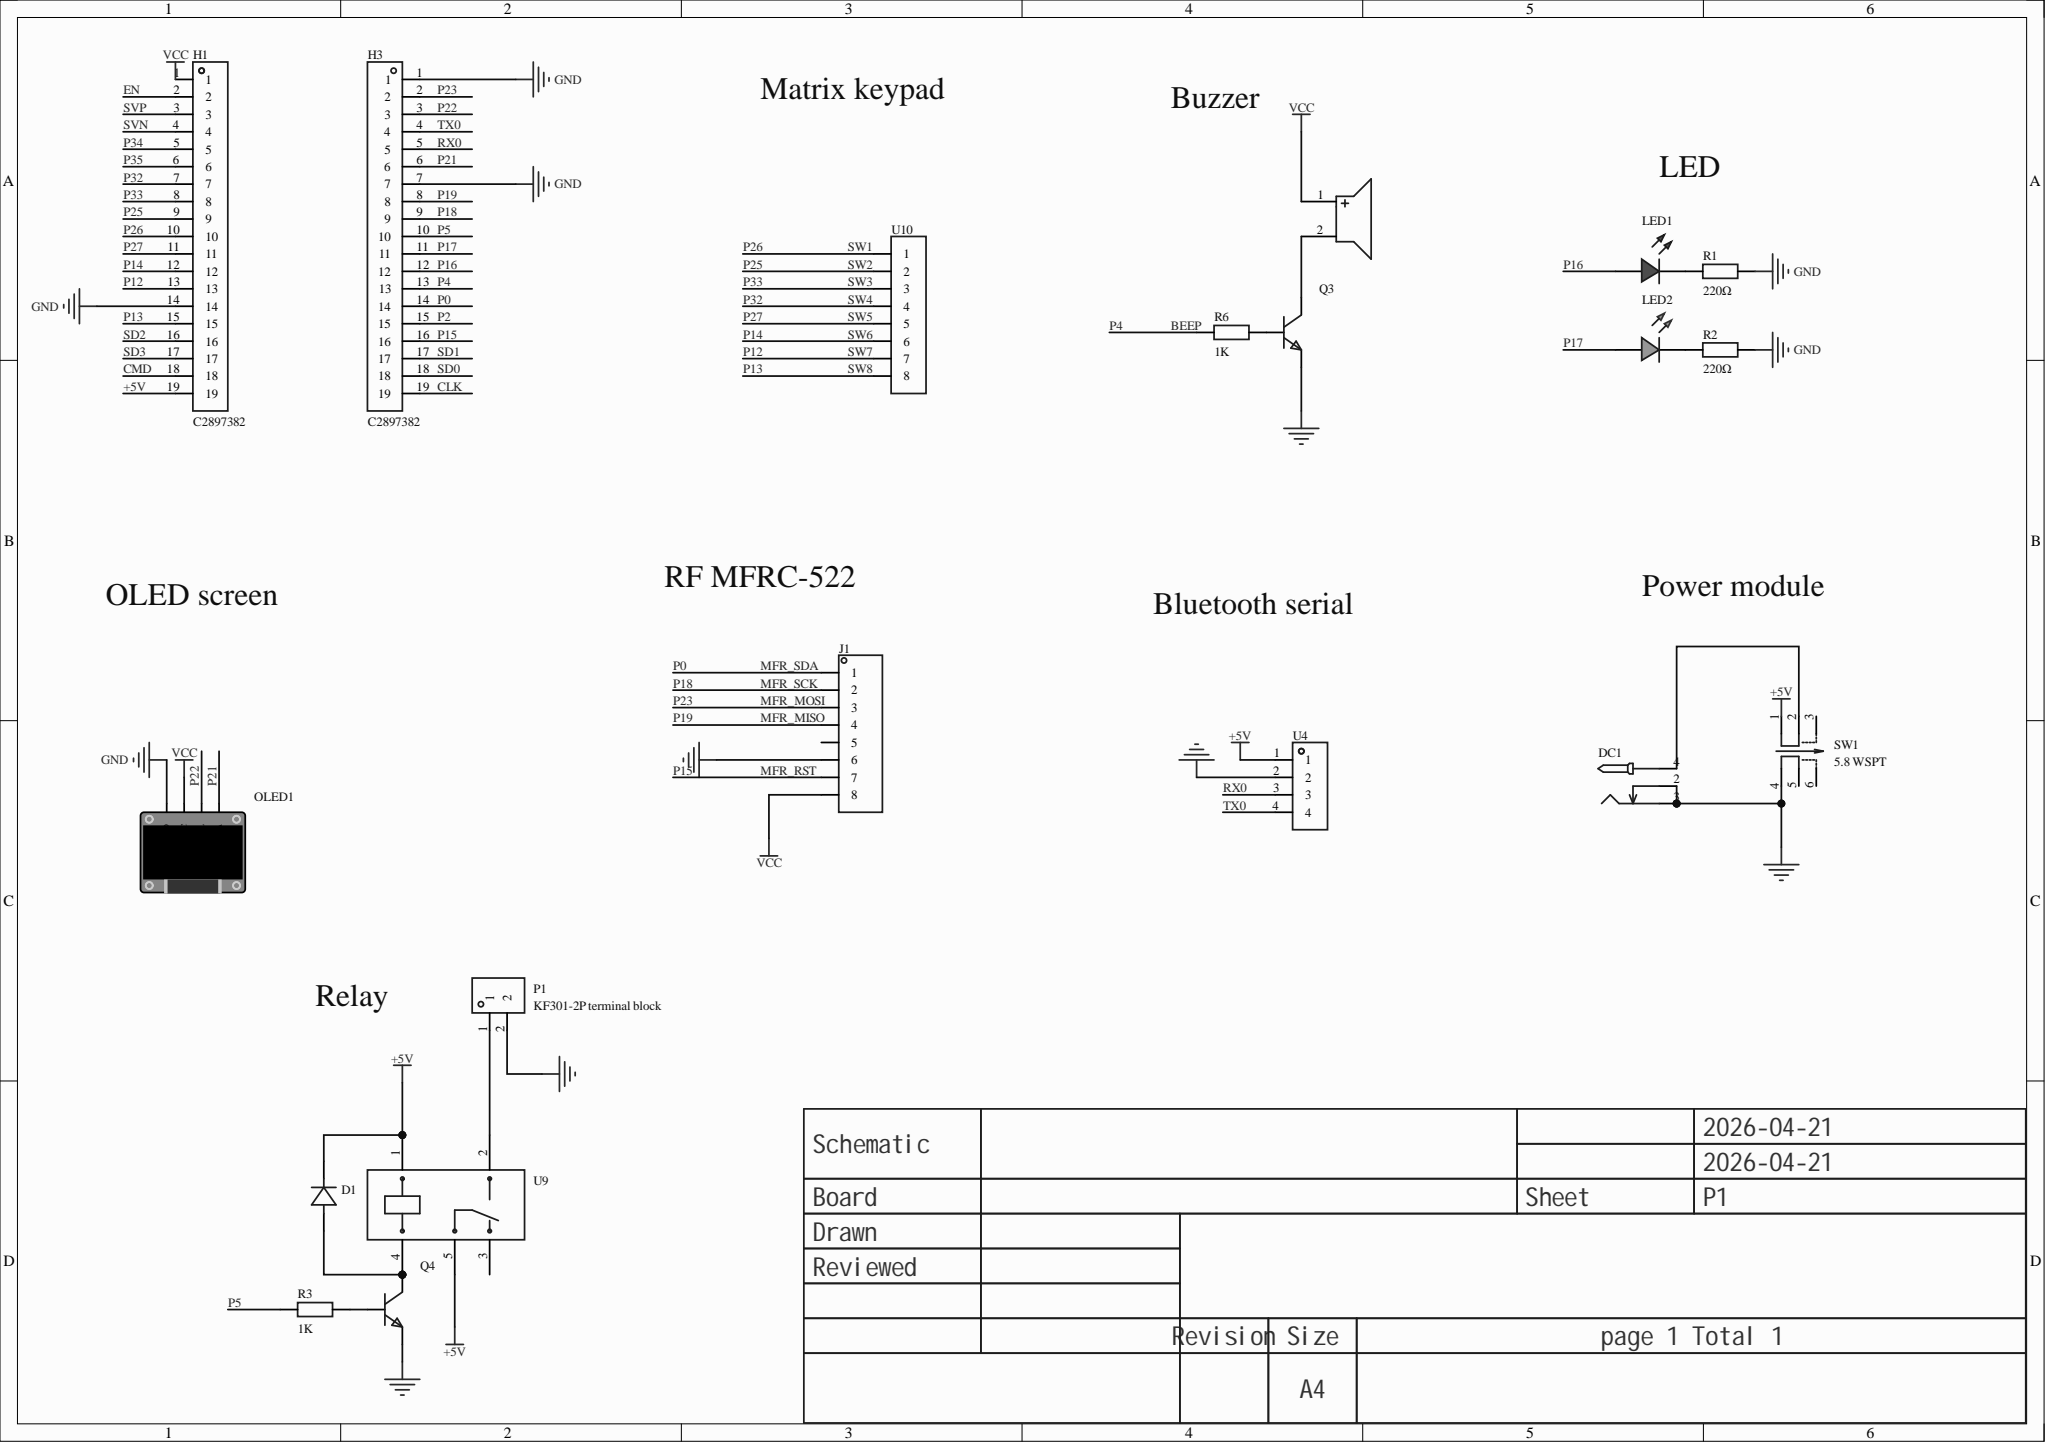Circuit board | Altium Designer | 20 parts | 32 nets
Bill of materials:
Comment,Description,Designator,Footprint,LibRef,Quantity
"2.7kHz","Drive mode: passive (external drive); type: electromagnetic; frequency: 2.7kHz; SPL: 85dB;","BUZZER1","BUZ-TH_BD9.0-P4.00-D0.6-FD","QMB-09B-03","1"
"","","D1","DO_1N4007","D_1N4007A","1"
"","","DC1","DC-2.0","DC-005_2.0","1"
"C2897382","","H1, H3","HDR-TH_19P-P2.54-V-F","HDR-F_2.54_1x19P","2"
"","","J1","HDR-TH_8P-P2.54-V-M","HDR-M_2.54_1x8P","1"
"","","LED1, LED2","LED_TH-3mm","LED_TH-R_3mm, LED_TH-G_3mm","2"
"","","OLED1","0.96OLED_4P","0.96OLED模块_4P","1"
"KF301-2P terminal block","","P1","CONN-TH_XY301V-A-5.0-2P","KF301-2P接线端子","1"
"","","Q3, Q4","S8050_TO_92","S8050_TO_NPN","2"
"220Ω","","R1, R2","Res_1/8W","Res_AXIAL-1/8W","2"
"1K","","R3, R6","Res_1/8W","Res_AXIAL-1/8W","2"
"5.8 WSPT","Circuit: DPDT; self-lock/no-lock: no-lock; mounting: through-hole; contact current: 100mA; rated voltage (AC): -; rated voltage (DC): 30V; with lamp: no; actuating force: 1.8N; mechanical life: 5 thousand cycles;","SW1","SW-TH_6P-L5.8-W5.8-P2.00-LS4.5-TL_K8-5851E-L1","5.8 WSPT","1"
"","","U4","HDR-TH_4P-P2.54-V-F","HDR-F_2.54_1x4P","1"
"SRD-12VDC-SL-C","Coil voltage: 12V; contact form: 1C (SPDT changeover); contact rating (resistive): -; max switching voltage: 250V@AC; max switching current: 15A;","U9","RELAY-TH_SRD-XXVDC-XL-C","SRD-12VDC-SL-C","1"
"","","U10","HDR-TH_8P-P2.54-V-F-1","HDR-F_2.54_1x8P","1"
Netlist (Protel format):
[
BUZZER1
BUZ-TH_BD9.0-P4.00-D0.6-FD
2.7kHz



]
[
D1
DO_1N4007




]
[
DC1
DC-2.0




]
[
H1
HDR-TH_19P-P2.54-V-F
C2897382



]
[
H3
HDR-TH_19P-P2.54-V-F
C2897382



]
[
J1
HDR-TH_8P-P2.54-V-M




]
[
LED1
LED_TH-3mm




]
[
LED2
LED_TH-3mm




]
[
OLED1
0.96OLED_4P




]
[
P1
CONN-TH_XY301V-A-5.0-2P
KF301-2P terminal block



]
[
Q3
S8050_TO_92




]
[
Q4
S8050_TO_92




]
[
R1
Res_1/8W
220Ω



]
[
R2
Res_1/8W
220Ω



]
[
R3
Res_1/8W
1K



]
[
R6
Res_1/8W
1K



]
[
SW1
SW-TH_6P-L5.8-W5.8-P2.00-LS4.5-TL_K8-5851E-L1
5.8 WSPT



]
[
U4
HDR-TH_4P-P2.54-V-F




]
[
U9
RELAY-TH_SRD-XXVDC-XL-C
SRD-12VDC-SL-C



]
[
U10
HDR-TH_8P-P2.54-V-F-1




]
(
VCC
BUZZER1-1
H1-1
J1-8
OLED1-2
)
(
TX0
H3-4
U4-4
)
(
RX0
H3-5
U4-3
)
(
P33
H1-8
U10-3
)
(
P32
H1-7
U10-4
)
(
P27
H1-11
U10-5
)
(
P26
H1-10
U10-1
)
(
P25
H1-9
U10-2
)
(
P22
H3-3
OLED1-3
)
(
P21
H3-6
OLED1-4
)
(
P17
H3-11
LED2-1
)
(
P16
H3-12
LED1-1
)
(
P14
H1-12
U10-6
)
(
P13
H1-15
U10-8
)
(
P12
H1-13
U10-7
)
(
P5
H3-10
R3-1
)
(
NetQ4_2
Q4-2
R3-2
)
(
NetQ3_2
Q3-2
R6-2
)
(
NetP1_1
P1-1
U9-2
)
(
NetLED2_2
LED2-2
R2-1
)
(
NetLED1_2
LED1-2
R1-1
)
(
NetDC1_4
DC1-4
SW1-2
)
(
NetD1_2
D1-2
Q4-3
U9-4
)
(
NetBUZZER1_2
BUZZER1-2
Q3-3
)
(
MFR_SDA
H3-14
J1-1
)
(
MFR_SCK
H3-9
J1-2
)
(
MFR_RST
H3-16
J1-7
)
(
MFR_MOSI
H3-2
J1-3
)
(
MFR_MISO
H3-8
J1-4
)
(
GND
DC1-2
DC1-3
H1-14
H3-1
H3-7
J1-6
OLED1-1
P1-2
Q3-1
Q4-1
R1-2
R2-2
SW1-4
U4-2
)
(
BEEP
H3-13
R6-1
)
(
+5V
D1-1
H1-19
SW1-1
U4-1
U9-1
U9-5
)